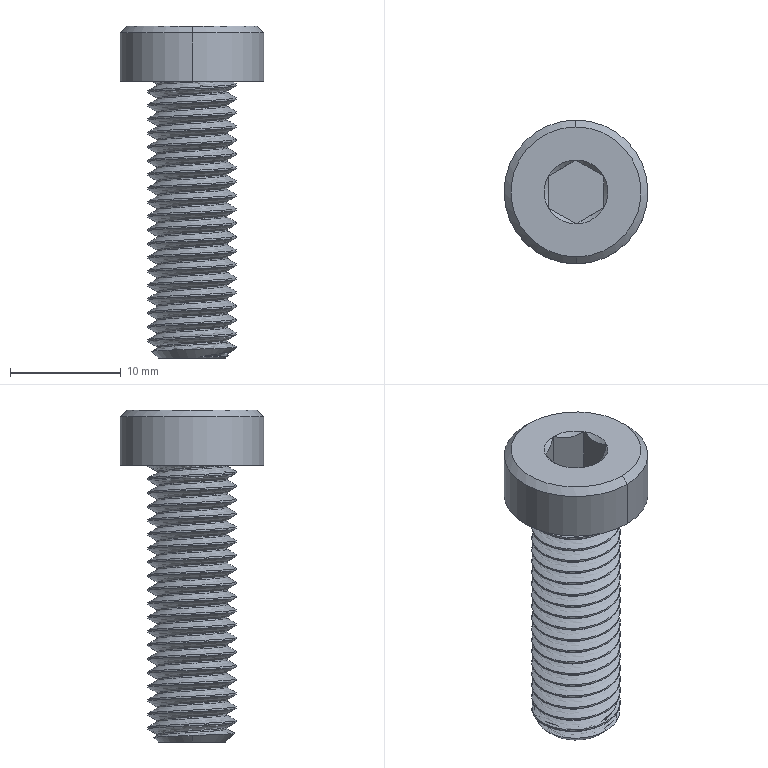Part | NX | features solid 2 | 1 solid | 66 faces | box 13 x 13 x 30 mm | volume 1587 mm3 | cylinder 42 | cone 11 | plane 10 | spline 3 | commonest cylinder face diameters 8 x40 13 x2